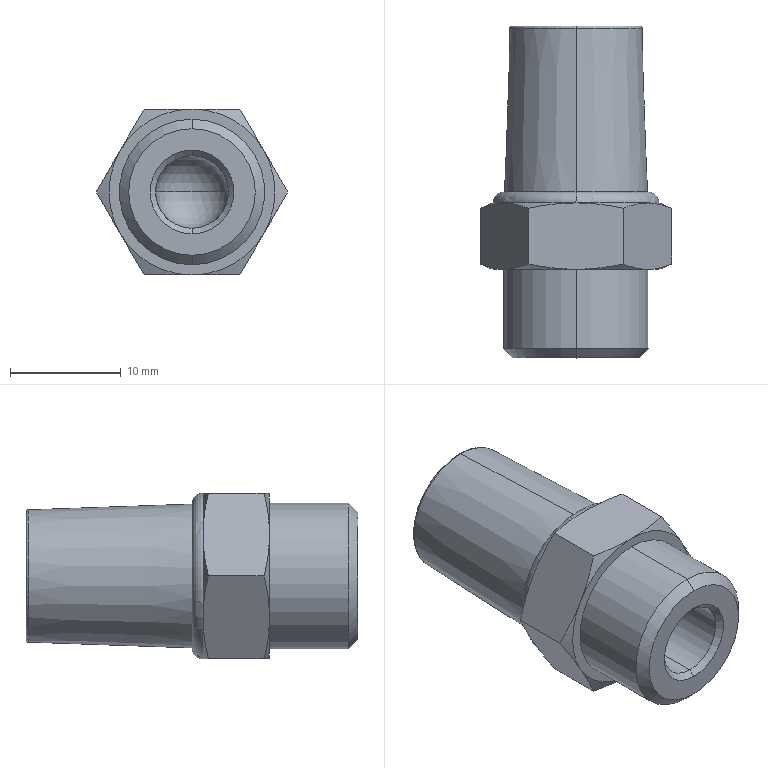Part | STEP file | BSL02 | 1 solid | 37 faces | box 17.321 x 30 x 15 mm | volume 3652 mm3 | cone 18 | plane 9 | torus 4 | cylinder 4 | sphere 2 | commonest cylinder face diameters 6.579 x2 13.157 x2